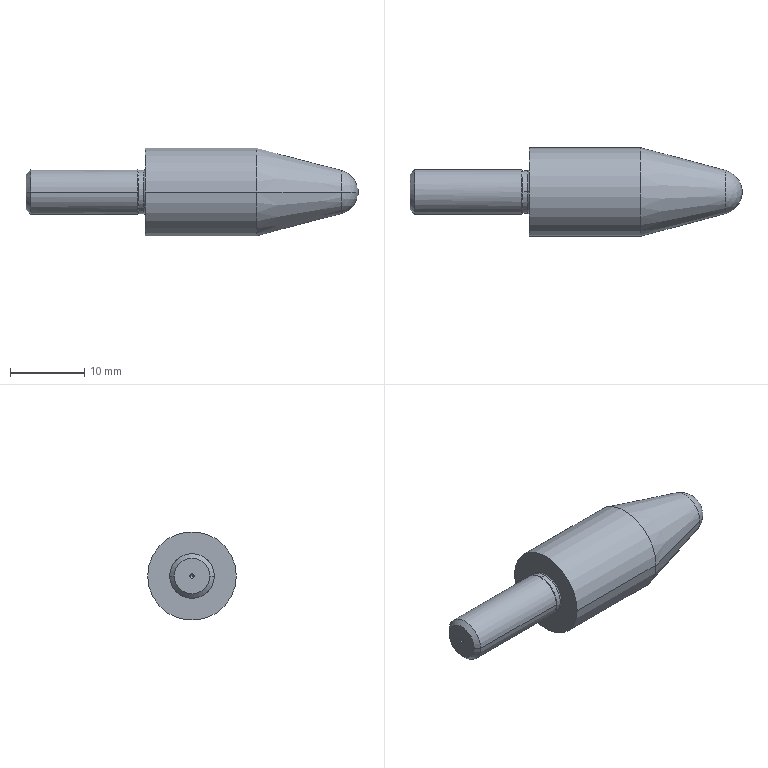Part | STEP file | FLNNA6_P11_9_B15_0_L10---2_FLNNA6-P11.9-B15.0-L10 | 1 solid | 22 faces | box 44.601 x 11.9 x 11.9 mm | volume 2879 mm3 | cone 8 | cylinder 6 | torus 4 | sphere 2 | plane 2 | commonest cylinder face diameters 5.8 x2 6 x2 11.9 x2